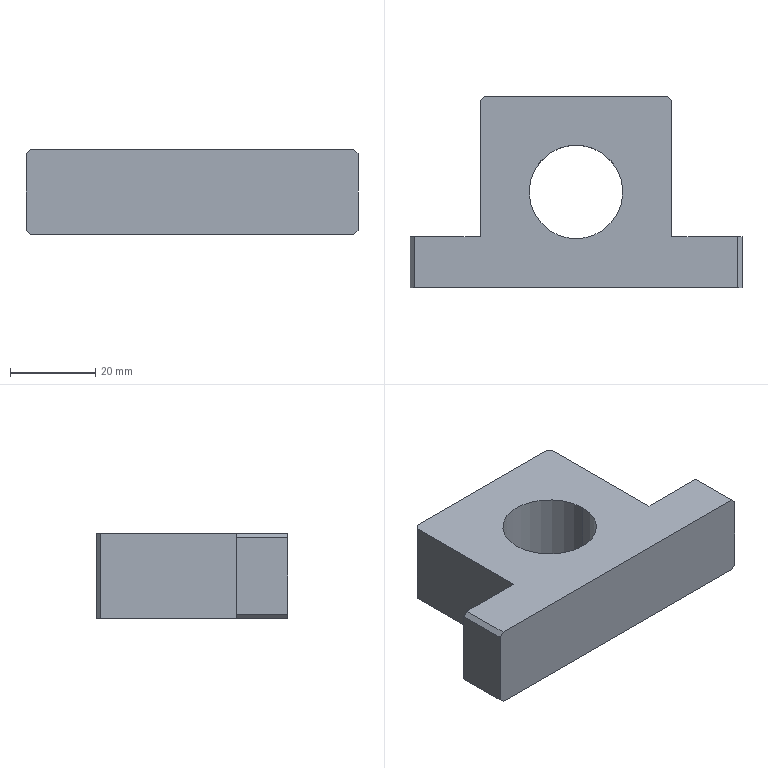Part | STEP file | 001-003-Shaft storage cylinder mounting seat | 1 solid | 18 faces | box 78 x 45 x 20 mm | volume 40773 mm3 | plane 16 | cylinder 2 | commonest cylinder face diameters 22 x2
STEP:
#1=CARTESIAN_POINT('',(0.,0.,0.));
#2=DIRECTION('',(0.,0.,1.));
#3=DIRECTION('',(1.,0.,0.));
#4=AXIS2_PLACEMENT_3D('',#1,#2,#3);
#5=CARTESIAN_POINT('',(11.,16.5,0.));
#6=VERTEX_POINT('',#5);
#7=CARTESIAN_POINT('',(11.,16.5,20.));
#8=VERTEX_POINT('',#7);
#9=CARTESIAN_POINT('',(11.,16.5,0.));
#10=DIRECTION('',(0.,0.,1.));
#11=VECTOR('',#10,1.);
#12=LINE('',#9,#11);
#13=CARTESIAN_POINT('',(0.,16.5,0.));
#14=DIRECTION('',(0.,0.,1.));
#15=DIRECTION('',(1.,0.,0.));
#16=AXIS2_PLACEMENT_3D('',#13,#14,#15);
#17=CYLINDRICAL_SURFACE('',#16,11.);
#18=CARTESIAN_POINT('',(6.283,0.));
#19=DIRECTION('',(0.,1.));
#20=VECTOR('',#19,1.);
#21=LINE('',#18,#20);
#22=(GEOMETRIC_REPRESENTATION_CONTEXT(2)PARAMETRIC_REPRESENTATION_CONTEXT()REPRESENTATION_CONTEXT('',''));
#23=DEFINITIONAL_REPRESENTATION('',(#21),#22);
#24=PCURVE('',#17,#23);
#25=CARTESIAN_POINT('',(0.,16.5,0.));
#26=DIRECTION('',(0.,0.,1.));
#27=DIRECTION('',(1.,0.,0.));
#28=AXIS2_PLACEMENT_3D('',#25,#26,#27);
#29=CYLINDRICAL_SURFACE('',#28,11.);
#30=CARTESIAN_POINT('',(0.,0.));
#31=DIRECTION('',(0.,1.));
#32=VECTOR('',#31,1.);
#33=LINE('',#30,#32);
#34=(GEOMETRIC_REPRESENTATION_CONTEXT(2)PARAMETRIC_REPRESENTATION_CONTEXT()REPRESENTATION_CONTEXT('',''));
#35=DEFINITIONAL_REPRESENTATION('',(#33),#34);
#36=PCURVE('',#29,#35);
#37=SURFACE_CURVE('',#12,(#24,#36),.PCURVE_S1.);
#38=EDGE_CURVE('',#6,#8,#37,.T.);
#39=ORIENTED_EDGE('',*,*,#38,.T.);
#40=CARTESIAN_POINT('',(-11.,16.5,20.));
#41=VERTEX_POINT('',#40);
#42=CARTESIAN_POINT('',(0.,16.5,20.));
#43=DIRECTION('',(0.,0.,1.));
#44=DIRECTION('',(1.,0.,0.));
#45=AXIS2_PLACEMENT_3D('',#42,#43,#44);
#46=CIRCLE('',#45,11.);
#47=CARTESIAN_POINT('',(0.,20.));
#48=DIRECTION('',(1.,0.));
#49=VECTOR('',#48,1.);
#50=LINE('',#47,#49);
#51=(GEOMETRIC_REPRESENTATION_CONTEXT(2)PARAMETRIC_REPRESENTATION_CONTEXT()REPRESENTATION_CONTEXT('',''));
#52=DEFINITIONAL_REPRESENTATION('',(#50),#51);
#53=PCURVE('',#17,#52);
#54=CARTESIAN_POINT('',(0.,0.,20.));
#55=DIRECTION('',(0.,0.,1.));
#56=DIRECTION('',(1.,0.,0.));
#57=AXIS2_PLACEMENT_3D('',#54,#55,#56);
#58=PLANE('',#57);
#59=CARTESIAN_POINT('',(0.,16.5));
#60=DIRECTION('',(1.,0.));
#61=AXIS2_PLACEMENT_2D('',#59,#60);
#62=CIRCLE('',#61,11.);
#63=(GEOMETRIC_REPRESENTATION_CONTEXT(2)PARAMETRIC_REPRESENTATION_CONTEXT()REPRESENTATION_CONTEXT('',''));
#64=DEFINITIONAL_REPRESENTATION('',(#62),#63);
#65=PCURVE('',#58,#64);
#66=SURFACE_CURVE('',#46,(#53,#65),.PCURVE_S1.);
#67=EDGE_CURVE('',#41,#8,#66,.T.);
#68=ORIENTED_EDGE('',*,*,#67,.F.);
#69=CARTESIAN_POINT('',(-11.,16.5,0.));
#70=VERTEX_POINT('',#69);
#71=CARTESIAN_POINT('',(-11.,16.5,0.));
#72=DIRECTION('',(0.,0.,1.));
#73=VECTOR('',#72,1.);
#74=LINE('',#71,#73);
#75=CARTESIAN_POINT('',(3.142,0.));
#76=DIRECTION('',(0.,1.));
#77=VECTOR('',#76,1.);
#78=LINE('',#75,#77);
#79=(GEOMETRIC_REPRESENTATION_CONTEXT(2)PARAMETRIC_REPRESENTATION_CONTEXT()REPRESENTATION_CONTEXT('',''));
#80=DEFINITIONAL_REPRESENTATION('',(#78),#79);
#81=PCURVE('',#17,#80);
#82=CARTESIAN_POINT('',(3.142,0.));
#83=DIRECTION('',(0.,1.));
#84=VECTOR('',#83,1.);
#85=LINE('',#82,#84);
#86=(GEOMETRIC_REPRESENTATION_CONTEXT(2)PARAMETRIC_REPRESENTATION_CONTEXT()REPRESENTATION_CONTEXT('',''));
#87=DEFINITIONAL_REPRESENTATION('',(#85),#86);
#88=PCURVE('',#29,#87);
#89=SURFACE_CURVE('',#74,(#81,#88),.PCURVE_S1.);
#90=EDGE_CURVE('',#70,#41,#89,.T.);
#91=ORIENTED_EDGE('',*,*,#90,.F.);
#92=CARTESIAN_POINT('',(0.,16.5,0.));
#93=DIRECTION('',(0.,0.,1.));
#94=DIRECTION('',(1.,0.,0.));
#95=AXIS2_PLACEMENT_3D('',#92,#93,#94);
#96=CIRCLE('',#95,11.);
#97=CARTESIAN_POINT('',(0.,0.));
#98=DIRECTION('',(1.,0.));
#99=VECTOR('',#98,1.);
#100=LINE('',#97,#99);
#101=(GEOMETRIC_REPRESENTATION_CONTEXT(2)PARAMETRIC_REPRESENTATION_CONTEXT()REPRESENTATION_CONTEXT('',''));
#102=DEFINITIONAL_REPRESENTATION('',(#100),#101);
#103=PCURVE('',#17,#102);
#104=CARTESIAN_POINT('',(0.,0.,0.));
#105=DIRECTION('',(0.,0.,1.));
#106=DIRECTION('',(1.,0.,0.));
#107=AXIS2_PLACEMENT_3D('',#104,#105,#106);
#108=PLANE('',#107);
#109=CARTESIAN_POINT('',(0.,16.5));
#110=DIRECTION('',(1.,0.));
#111=AXIS2_PLACEMENT_2D('',#109,#110);
#112=CIRCLE('',#111,11.);
#113=(GEOMETRIC_REPRESENTATION_CONTEXT(2)PARAMETRIC_REPRESENTATION_CONTEXT()REPRESENTATION_CONTEXT('',''));
#114=DEFINITIONAL_REPRESENTATION('',(#112),#113);
#115=PCURVE('',#108,#114);
#116=SURFACE_CURVE('',#96,(#103,#115),.PCURVE_S1.);
#117=EDGE_CURVE('',#70,#6,#116,.T.);
#118=ORIENTED_EDGE('',*,*,#117,.T.);
#119=EDGE_LOOP('',(#39,#68,#91,#118));
#120=FACE_BOUND('',#119,.F.);
#121=ADVANCED_FACE('',(#120),#17,.F.);
#122=CARTESIAN_POINT('',(39.,6.,19.));
#123=VERTEX_POINT('',#122);
#124=CARTESIAN_POINT('',(39.,6.,1.));
#125=VERTEX_POINT('',#124);
#126=CARTESIAN_POINT('',(39.,6.,20.));
#127=DIRECTION('',(0.,0.,-1.));
#128=VECTOR('',#127,1.);
#129=LINE('',#126,#128);
#130=CARTESIAN_POINT('',(22.5,6.,20.));
#131=DIRECTION('',(0.,-1.,0.));
#132=DIRECTION('',(1.,0.,0.));
#133=AXIS2_PLACEMENT_3D('',#130,#131,#132);
#134=PLANE('',#133);
#135=CARTESIAN_POINT('',(16.5,0.));
#136=DIRECTION('',(0.,-1.));
#137=VECTOR('',#136,1.);
#138=LINE('',#135,#137);
#139=(GEOMETRIC_REPRESENTATION_CONTEXT(2)PARAMETRIC_REPRESENTATION_CONTEXT()REPRESENTATION_CONTEXT('',''));
#140=DEFINITIONAL_REPRESENTATION('',(#138),#139);
#141=PCURVE('',#134,#140);
#142=CARTESIAN_POINT('',(39.,-6.,20.));
#143=DIRECTION('',(-1.,0.,0.));
#144=DIRECTION('',(0.,0.,1.));
#145=AXIS2_PLACEMENT_3D('',#142,#143,#144);
#146=PLANE('',#145);
#147=CARTESIAN_POINT('',(0.,12.));
#148=DIRECTION('',(-1.,0.));
#149=VECTOR('',#148,1.);
#150=LINE('',#147,#149);
#151=(GEOMETRIC_REPRESENTATION_CONTEXT(2)PARAMETRIC_REPRESENTATION_CONTEXT()REPRESENTATION_CONTEXT('',''));
#152=DEFINITIONAL_REPRESENTATION('',(#150),#151);
#153=PCURVE('',#146,#152);
#154=SURFACE_CURVE('',#129,(#141,#153),.PCURVE_S1.);
#155=EDGE_CURVE('',#123,#125,#154,.T.);
#156=ORIENTED_EDGE('',*,*,#155,.T.);
#157=CARTESIAN_POINT('',(38.,6.,0.));
#158=VERTEX_POINT('',#157);
#159=CARTESIAN_POINT('',(39.,6.,1.));
#160=DIRECTION('',(-0.7071,0.,-0.7071));
#161=VECTOR('',#160,1.);
#162=LINE('',#159,#161);
#163=CARTESIAN_POINT('',(16.5,-19.));
#164=DIRECTION('',(-0.7071,-0.7071));
#165=VECTOR('',#164,1.);
#166=LINE('',#163,#165);
#167=(GEOMETRIC_REPRESENTATION_CONTEXT(2)PARAMETRIC_REPRESENTATION_CONTEXT()REPRESENTATION_CONTEXT('',''));
#168=DEFINITIONAL_REPRESENTATION('',(#166),#167);
#169=PCURVE('',#134,#168);
#170=CARTESIAN_POINT('',(39.,-6.,1.));
#171=DIRECTION('',(-0.7071,0.,0.7071));
#172=DIRECTION('',(0.,1.,0.));
#173=AXIS2_PLACEMENT_3D('',#170,#171,#172);
#174=PLANE('',#173);
#175=CARTESIAN_POINT('',(12.,0.));
#176=DIRECTION('',(0.,1.));
#177=VECTOR('',#176,1.);
#178=LINE('',#175,#177);
#179=(GEOMETRIC_REPRESENTATION_CONTEXT(2)PARAMETRIC_REPRESENTATION_CONTEXT()REPRESENTATION_CONTEXT('',''));
#180=DEFINITIONAL_REPRESENTATION('',(#178),#179);
#181=PCURVE('',#174,#180);
#182=SURFACE_CURVE('',#162,(#169,#181),.PCURVE_S1.);
#183=EDGE_CURVE('',#125,#158,#182,.T.);
#184=ORIENTED_EDGE('',*,*,#183,.T.);
#185=CARTESIAN_POINT('',(22.5,6.,0.));
#186=VERTEX_POINT('',#185);
#187=CARTESIAN_POINT('',(22.5,6.,0.));
#188=DIRECTION('',(-1.,0.,0.));
#189=VECTOR('',#188,1.);
#190=LINE('',#187,#189);
#191=CARTESIAN_POINT('',(0.,-20.));
#192=DIRECTION('',(-1.,0.));
#193=VECTOR('',#192,1.);
#194=LINE('',#191,#193);
#195=(GEOMETRIC_REPRESENTATION_CONTEXT(2)PARAMETRIC_REPRESENTATION_CONTEXT()REPRESENTATION_CONTEXT('',''));
#196=DEFINITIONAL_REPRESENTATION('',(#194),#195);
#197=PCURVE('',#134,#196);
#198=CARTESIAN_POINT('',(22.5,6.));
#199=DIRECTION('',(-1.,0.));
#200=VECTOR('',#199,1.);
#201=LINE('',#198,#200);
#202=(GEOMETRIC_REPRESENTATION_CONTEXT(2)PARAMETRIC_REPRESENTATION_CONTEXT()REPRESENTATION_CONTEXT('',''));
#203=DEFINITIONAL_REPRESENTATION('',(#201),#202);
#204=PCURVE('',#108,#203);
#205=SURFACE_CURVE('',#190,(#197,#204),.PCURVE_S1.);
#206=EDGE_CURVE('',#158,#186,#205,.T.);
#207=ORIENTED_EDGE('',*,*,#206,.T.);
#208=CARTESIAN_POINT('',(22.5,6.,20.));
#209=VERTEX_POINT('',#208);
#210=CARTESIAN_POINT('',(22.5,6.,20.));
#211=DIRECTION('',(0.,0.,-1.));
#212=VECTOR('',#211,1.);
#213=LINE('',#210,#212);
#214=CARTESIAN_POINT('',(0.,0.));
#215=DIRECTION('',(0.,-1.));
#216=VECTOR('',#215,1.);
#217=LINE('',#214,#216);
#218=(GEOMETRIC_REPRESENTATION_CONTEXT(2)PARAMETRIC_REPRESENTATION_CONTEXT()REPRESENTATION_CONTEXT('',''));
#219=DEFINITIONAL_REPRESENTATION('',(#217),#218);
#220=PCURVE('',#134,#219);
#221=CARTESIAN_POINT('',(22.5,6.,20.));
#222=DIRECTION('',(-1.,0.,0.));
#223=DIRECTION('',(0.,-1.,0.));
#224=AXIS2_PLACEMENT_3D('',#221,#222,#223);
#225=PLANE('',#224);
#226=CARTESIAN_POINT('',(0.,0.));
#227=DIRECTION('',(0.,-1.));
#228=VECTOR('',#227,1.);
#229=LINE('',#226,#228);
#230=(GEOMETRIC_REPRESENTATION_CONTEXT(2)PARAMETRIC_REPRESENTATION_CONTEXT()REPRESENTATION_CONTEXT('',''));
#231=DEFINITIONAL_REPRESENTATION('',(#229),#230);
#232=PCURVE('',#225,#231);
#233=SURFACE_CURVE('',#213,(#220,#232),.PCURVE_S1.);
#234=EDGE_CURVE('',#209,#186,#233,.T.);
#235=ORIENTED_EDGE('',*,*,#234,.F.);
#236=CARTESIAN_POINT('',(38.,6.,20.));
#237=VERTEX_POINT('',#236);
#238=CARTESIAN_POINT('',(22.5,6.,20.));
#239=DIRECTION('',(-1.,0.,0.));
#240=VECTOR('',#239,1.);
#241=LINE('',#238,#240);
#242=CARTESIAN_POINT('',(0.,0.));
#243=DIRECTION('',(-1.,0.));
#244=VECTOR('',#243,1.);
#245=LINE('',#242,#244);
#246=(GEOMETRIC_REPRESENTATION_CONTEXT(2)PARAMETRIC_REPRESENTATION_CONTEXT()REPRESENTATION_CONTEXT('',''));
#247=DEFINITIONAL_REPRESENTATION('',(#245),#246);
#248=PCURVE('',#134,#247);
#249=CARTESIAN_POINT('',(22.5,6.));
#250=DIRECTION('',(-1.,0.));
#251=VECTOR('',#250,1.);
#252=LINE('',#249,#251);
#253=(GEOMETRIC_REPRESENTATION_CONTEXT(2)PARAMETRIC_REPRESENTATION_CONTEXT()REPRESENTATION_CONTEXT('',''));
#254=DEFINITIONAL_REPRESENTATION('',(#252),#253);
#255=PCURVE('',#58,#254);
#256=SURFACE_CURVE('',#241,(#248,#255),.PCURVE_S1.);
#257=EDGE_CURVE('',#237,#209,#256,.T.);
#258=ORIENTED_EDGE('',*,*,#257,.F.);
#259=CARTESIAN_POINT('',(38.,6.,20.));
#260=DIRECTION('',(0.7071,0.,-0.7071));
#261=VECTOR('',#260,1.);
#262=LINE('',#259,#261);
#263=CARTESIAN_POINT('',(15.5,0.));
#264=DIRECTION('',(0.7071,-0.7071));
#265=VECTOR('',#264,1.);
#266=LINE('',#263,#265);
#267=(GEOMETRIC_REPRESENTATION_CONTEXT(2)PARAMETRIC_REPRESENTATION_CONTEXT()REPRESENTATION_CONTEXT('',''));
#268=DEFINITIONAL_REPRESENTATION('',(#266),#267);
#269=PCURVE('',#134,#268);
#270=CARTESIAN_POINT('',(38.,0.,20.));
#271=DIRECTION('',(0.7071,0.,0.7071));
#272=DIRECTION('',(0.,-1.,0.));
#273=AXIS2_PLACEMENT_3D('',#270,#271,#272);
#274=PLANE('',#273);
#275=CARTESIAN_POINT('',(-6.,0.));
#276=DIRECTION('',(0.,1.));
#277=VECTOR('',#276,1.);
#278=LINE('',#275,#277);
#279=(GEOMETRIC_REPRESENTATION_CONTEXT(2)PARAMETRIC_REPRESENTATION_CONTEXT()REPRESENTATION_CONTEXT('',''));
#280=DEFINITIONAL_REPRESENTATION('',(#278),#279);
#281=PCURVE('',#274,#280);
#282=SURFACE_CURVE('',#262,(#269,#281),.PCURVE_S1.);
#283=EDGE_CURVE('',#237,#123,#282,.T.);
#284=ORIENTED_EDGE('',*,*,#283,.T.);
#285=EDGE_LOOP('',(#156,#184,#207,#235,#258,#284));
#286=FACE_BOUND('',#285,.T.);
#287=ADVANCED_FACE('',(#286),#134,.F.);
#288=CARTESIAN_POINT('',(22.5,38.,0.));
#289=VERTEX_POINT('',#288);
#290=CARTESIAN_POINT('',(22.5,6.,0.));
#291=DIRECTION('',(0.,1.,0.));
#292=VECTOR('',#291,1.);
#293=LINE('',#290,#292);
#294=CARTESIAN_POINT('',(0.,-20.));
#295=DIRECTION('',(-1.,0.));
#296=VECTOR('',#295,1.);
#297=LINE('',#294,#296);
#298=(GEOMETRIC_REPRESENTATION_CONTEXT(2)PARAMETRIC_REPRESENTATION_CONTEXT()REPRESENTATION_CONTEXT('',''));
#299=DEFINITIONAL_REPRESENTATION('',(#297),#298);
#300=PCURVE('',#225,#299);
#301=CARTESIAN_POINT('',(22.5,6.));
#302=DIRECTION('',(0.,1.));
#303=VECTOR('',#302,1.);
#304=LINE('',#301,#303);
#305=(GEOMETRIC_REPRESENTATION_CONTEXT(2)PARAMETRIC_REPRESENTATION_CONTEXT()REPRESENTATION_CONTEXT('',''));
#306=DEFINITIONAL_REPRESENTATION('',(#304),#305);
#307=PCURVE('',#108,#306);
#308=SURFACE_CURVE('',#293,(#300,#307),.PCURVE_S1.);
#309=EDGE_CURVE('',#186,#289,#308,.T.);
#310=ORIENTED_EDGE('',*,*,#309,.T.);
#311=CARTESIAN_POINT('',(22.5,38.,20.));
#312=VERTEX_POINT('',#311);
#313=CARTESIAN_POINT('',(22.5,38.,20.));
#314=DIRECTION('',(0.,0.,1.));
#315=VECTOR('',#314,1.);
#316=LINE('',#313,#315);
#317=CARTESIAN_POINT('',(-32.,0.));
#318=DIRECTION('',(0.,1.));
#319=VECTOR('',#318,1.);
#320=LINE('',#317,#319);
#321=(GEOMETRIC_REPRESENTATION_CONTEXT(2)PARAMETRIC_REPRESENTATION_CONTEXT()REPRESENTATION_CONTEXT('',''));
#322=DEFINITIONAL_REPRESENTATION('',(#320),#321);
#323=PCURVE('',#225,#322);
#324=CARTESIAN_POINT('',(21.5,39.,20.));
#325=DIRECTION('',(-0.7071,-0.7071,0.));
#326=DIRECTION('',(0.,0.,-1.));
#327=AXIS2_PLACEMENT_3D('',#324,#325,#326);
#328=PLANE('',#327);
#329=CARTESIAN_POINT('',(0.,1.414));
#330=DIRECTION('',(-1.,0.));
#331=VECTOR('',#330,1.);
#332=LINE('',#329,#331);
#333=(GEOMETRIC_REPRESENTATION_CONTEXT(2)PARAMETRIC_REPRESENTATION_CONTEXT()REPRESENTATION_CONTEXT('',''));
#334=DEFINITIONAL_REPRESENTATION('',(#332),#333);
#335=PCURVE('',#328,#334);
#336=SURFACE_CURVE('',#316,(#323,#335),.PCURVE_S1.);
#337=EDGE_CURVE('',#289,#312,#336,.T.);
#338=ORIENTED_EDGE('',*,*,#337,.T.);
#339=CARTESIAN_POINT('',(22.5,6.,20.));
#340=DIRECTION('',(0.,1.,0.));
#341=VECTOR('',#340,1.);
#342=LINE('',#339,#341);
#343=CARTESIAN_POINT('',(0.,0.));
#344=DIRECTION('',(-1.,0.));
#345=VECTOR('',#344,1.);
#346=LINE('',#343,#345);
#347=(GEOMETRIC_REPRESENTATION_CONTEXT(2)PARAMETRIC_REPRESENTATION_CONTEXT()REPRESENTATION_CONTEXT('',''));
#348=DEFINITIONAL_REPRESENTATION('',(#346),#347);
#349=PCURVE('',#225,#348);
#350=CARTESIAN_POINT('',(22.5,6.));
#351=DIRECTION('',(0.,1.));
#352=VECTOR('',#351,1.);
#353=LINE('',#350,#352);
#354=(GEOMETRIC_REPRESENTATION_CONTEXT(2)PARAMETRIC_REPRESENTATION_CONTEXT()REPRESENTATION_CONTEXT('',''));
#355=DEFINITIONAL_REPRESENTATION('',(#353),#354);
#356=PCURVE('',#58,#355);
#357=SURFACE_CURVE('',#342,(#349,#356),.PCURVE_S1.);
#358=EDGE_CURVE('',#209,#312,#357,.T.);
#359=ORIENTED_EDGE('',*,*,#358,.F.);
#360=ORIENTED_EDGE('',*,*,#234,.T.);
#361=EDGE_LOOP('',(#310,#338,#359,#360));
#362=FACE_BOUND('',#361,.T.);
#363=ADVANCED_FACE('',(#362),#225,.F.);
#364=CARTESIAN_POINT('',(21.5,39.,20.));
#365=VERTEX_POINT('',#364);
#366=CARTESIAN_POINT('',(-21.5,39.,20.));
#367=VERTEX_POINT('',#366);
#368=CARTESIAN_POINT('',(-22.5,39.,20.));
#369=DIRECTION('',(-1.,0.,0.));
#370=VECTOR('',#369,1.);
#371=LINE('',#368,#370);
#372=CARTESIAN_POINT('',(-22.5,39.,20.));
#373=DIRECTION('',(0.,-1.,0.));
#374=DIRECTION('',(1.,0.,0.));
#375=AXIS2_PLACEMENT_3D('',#372,#373,#374);
#376=PLANE('',#375);
#377=CARTESIAN_POINT('',(0.,0.));
#378=DIRECTION('',(-1.,0.));
#379=VECTOR('',#378,1.);
#380=LINE('',#377,#379);
#381=(GEOMETRIC_REPRESENTATION_CONTEXT(2)PARAMETRIC_REPRESENTATION_CONTEXT()REPRESENTATION_CONTEXT('',''));
#382=DEFINITIONAL_REPRESENTATION('',(#380),#381);
#383=PCURVE('',#376,#382);
#384=CARTESIAN_POINT('',(-22.5,39.));
#385=DIRECTION('',(-1.,0.));
#386=VECTOR('',#385,1.);
#387=LINE('',#384,#386);
#388=(GEOMETRIC_REPRESENTATION_CONTEXT(2)PARAMETRIC_REPRESENTATION_CONTEXT()REPRESENTATION_CONTEXT('',''));
#389=DEFINITIONAL_REPRESENTATION('',(#387),#388);
#390=PCURVE('',#58,#389);
#391=SURFACE_CURVE('',#371,(#383,#390),.PCURVE_S1.);
#392=EDGE_CURVE('',#365,#367,#391,.T.);
#393=ORIENTED_EDGE('',*,*,#392,.F.);
#394=CARTESIAN_POINT('',(21.5,39.,0.));
#395=VERTEX_POINT('',#394);
#396=CARTESIAN_POINT('',(21.5,39.,20.));
#397=DIRECTION('',(0.,0.,-1.));
#398=VECTOR('',#397,1.);
#399=LINE('',#396,#398);
#400=CARTESIAN_POINT('',(44.,0.));
#401=DIRECTION('',(0.,-1.));
#402=VECTOR('',#401,1.);
#403=LINE('',#400,#402);
#404=(GEOMETRIC_REPRESENTATION_CONTEXT(2)PARAMETRIC_REPRESENTATION_CONTEXT()REPRESENTATION_CONTEXT('',''));
#405=DEFINITIONAL_REPRESENTATION('',(#403),#404);
#406=PCURVE('',#376,#405);
#407=CARTESIAN_POINT('',(0.,0.));
#408=DIRECTION('',(1.,0.));
#409=VECTOR('',#408,1.);
#410=LINE('',#407,#409);
#411=(GEOMETRIC_REPRESENTATION_CONTEXT(2)PARAMETRIC_REPRESENTATION_CONTEXT()REPRESENTATION_CONTEXT('',''));
#412=DEFINITIONAL_REPRESENTATION('',(#410),#411);
#413=PCURVE('',#328,#412);
#414=SURFACE_CURVE('',#399,(#406,#413),.PCURVE_S1.);
#415=EDGE_CURVE('',#365,#395,#414,.T.);
#416=ORIENTED_EDGE('',*,*,#415,.T.);
#417=CARTESIAN_POINT('',(-21.5,39.,0.));
#418=VERTEX_POINT('',#417);
#419=CARTESIAN_POINT('',(-22.5,39.,0.));
#420=DIRECTION('',(-1.,0.,0.));
#421=VECTOR('',#420,1.);
#422=LINE('',#419,#421);
#423=CARTESIAN_POINT('',(0.,-20.));
#424=DIRECTION('',(-1.,0.));
#425=VECTOR('',#424,1.);
#426=LINE('',#423,#425);
#427=(GEOMETRIC_REPRESENTATION_CONTEXT(2)PARAMETRIC_REPRESENTATION_CONTEXT()REPRESENTATION_CONTEXT('',''));
#428=DEFINITIONAL_REPRESENTATION('',(#426),#427);
#429=PCURVE('',#376,#428);
#430=CARTESIAN_POINT('',(-22.5,39.));
#431=DIRECTION('',(-1.,0.));
#432=VECTOR('',#431,1.);
#433=LINE('',#430,#432);
#434=(GEOMETRIC_REPRESENTATION_CONTEXT(2)PARAMETRIC_REPRESENTATION_CONTEXT()REPRESENTATION_CONTEXT('',''));
#435=DEFINITIONAL_REPRESENTATION('',(#433),#434);
#436=PCURVE('',#108,#435);
#437=SURFACE_CURVE('',#422,(#429,#436),.PCURVE_S1.);
#438=EDGE_CURVE('',#395,#418,#437,.T.);
#439=ORIENTED_EDGE('',*,*,#438,.T.);
#440=CARTESIAN_POINT('',(-21.5,39.,20.));
#441=DIRECTION('',(0.,0.,1.));
#442=VECTOR('',#441,1.);
#443=LINE('',#440,#442);
#444=CARTESIAN_POINT('',(1.,0.));
#445=DIRECTION('',(0.,1.));
#446=VECTOR('',#445,1.);
#447=LINE('',#444,#446);
#448=(GEOMETRIC_REPRESENTATION_CONTEXT(2)PARAMETRIC_REPRESENTATION_CONTEXT()REPRESENTATION_CONTEXT('',''));
#449=DEFINITIONAL_REPRESENTATION('',(#447),#448);
#450=PCURVE('',#376,#449);
#451=CARTESIAN_POINT('',(-22.5,38.,20.));
#452=DIRECTION('',(0.7071,-0.7071,0.));
#453=DIRECTION('',(0.,0.,-1.));
#454=AXIS2_PLACEMENT_3D('',#451,#452,#453);
#455=PLANE('',#454);
#456=CARTESIAN_POINT('',(0.,1.414));
#457=DIRECTION('',(-1.,0.));
#458=VECTOR('',#457,1.);
#459=LINE('',#456,#458);
#460=(GEOMETRIC_REPRESENTATION_CONTEXT(2)PARAMETRIC_REPRESENTATION_CONTEXT()REPRESENTATION_CONTEXT('',''));
#461=DEFINITIONAL_REPRESENTATION('',(#459),#460);
#462=PCURVE('',#455,#461);
#463=SURFACE_CURVE('',#443,(#450,#462),.PCURVE_S1.);
#464=EDGE_CURVE('',#418,#367,#463,.T.);
#465=ORIENTED_EDGE('',*,*,#464,.T.);
#466=EDGE_LOOP('',(#393,#416,#439,#465));
#467=FACE_BOUND('',#466,.T.);
#468=ADVANCED_FACE('',(#467),#376,.F.);
#469=CARTESIAN_POINT('',(-22.5,38.,20.));
#470=VERTEX_POINT('',#469);
#471=CARTESIAN_POINT('',(-22.5,6.,20.));
#472=VERTEX_POINT('',#471);
#473=CARTESIAN_POINT('',(-22.5,6.,20.));
#474=DIRECTION('',(0.,-1.,0.));
#475=VECTOR('',#474,1.);
#476=LINE('',#473,#475);
#477=CARTESIAN_POINT('',(-22.5,6.,20.));
#478=DIRECTION('',(1.,0.,0.));
#479=DIRECTION('',(0.,0.,-1.));
#480=AXIS2_PLACEMENT_3D('',#477,#478,#479);
#481=PLANE('',#480);
#482=CARTESIAN_POINT('',(0.,0.));
#483=DIRECTION('',(0.,-1.));
#484=VECTOR('',#483,1.);
#485=LINE('',#482,#484);
#486=(GEOMETRIC_REPRESENTATION_CONTEXT(2)PARAMETRIC_REPRESENTATION_CONTEXT()REPRESENTATION_CONTEXT('',''));
#487=DEFINITIONAL_REPRESENTATION('',(#485),#486);
#488=PCURVE('',#481,#487);
#489=CARTESIAN_POINT('',(-22.5,6.));
#490=DIRECTION('',(0.,-1.));
#491=VECTOR('',#490,1.);
#492=LINE('',#489,#491);
#493=(GEOMETRIC_REPRESENTATION_CONTEXT(2)PARAMETRIC_REPRESENTATION_CONTEXT()REPRESENTATION_CONTEXT('',''));
#494=DEFINITIONAL_REPRESENTATION('',(#492),#493);
#495=PCURVE('',#58,#494);
#496=SURFACE_CURVE('',#476,(#488,#495),.PCURVE_S1.);
#497=EDGE_CURVE('',#470,#472,#496,.T.);
#498=ORIENTED_EDGE('',*,*,#497,.F.);
#499=CARTESIAN_POINT('',(-22.5,38.,0.));
#500=VERTEX_POINT('',#499);
#501=CARTESIAN_POINT('',(-22.5,38.,20.));
#502=DIRECTION('',(0.,0.,-1.));
#503=VECTOR('',#502,1.);
#504=LINE('',#501,#503);
#505=CARTESIAN_POINT('',(0.,32.));
#506=DIRECTION('',(1.,0.));
#507=VECTOR('',#506,1.);
#508=LINE('',#505,#507);
#509=(GEOMETRIC_REPRESENTATION_CONTEXT(2)PARAMETRIC_REPRESENTATION_CONTEXT()REPRESENTATION_CONTEXT('',''));
#510=DEFINITIONAL_REPRESENTATION('',(#508),#509);
#511=PCURVE('',#481,#510);
#512=CARTESIAN_POINT('',(0.,0.));
#513=DIRECTION('',(1.,0.));
#514=VECTOR('',#513,1.);
#515=LINE('',#512,#514);
#516=(GEOMETRIC_REPRESENTATION_CONTEXT(2)PARAMETRIC_REPRESENTATION_CONTEXT()REPRESENTATION_CONTEXT('',''));
#517=DEFINITIONAL_REPRESENTATION('',(#515),#516);
#518=PCURVE('',#455,#517);
#519=SURFACE_CURVE('',#504,(#511,#518),.PCURVE_S1.);
#520=EDGE_CURVE('',#470,#500,#519,.T.);
#521=ORIENTED_EDGE('',*,*,#520,.T.);
#522=CARTESIAN_POINT('',(-22.5,6.,0.));
#523=VERTEX_POINT('',#522);
#524=CARTESIAN_POINT('',(-22.5,6.,0.));
#525=DIRECTION('',(0.,-1.,0.));
#526=VECTOR('',#525,1.);
#527=LINE('',#524,#526);
#528=CARTESIAN_POINT('',(20.,0.));
#529=DIRECTION('',(0.,-1.));
#530=VECTOR('',#529,1.);
#531=LINE('',#528,#530);
#532=(GEOMETRIC_REPRESENTATION_CONTEXT(2)PARAMETRIC_REPRESENTATION_CONTEXT()REPRESENTATION_CONTEXT('',''));
#533=DEFINITIONAL_REPRESENTATION('',(#531),#532);
#534=PCURVE('',#481,#533);
#535=CARTESIAN_POINT('',(-22.5,6.));
#536=DIRECTION('',(0.,-1.));
#537=VECTOR('',#536,1.);
#538=LINE('',#535,#537);
#539=(GEOMETRIC_REPRESENTATION_CONTEXT(2)PARAMETRIC_REPRESENTATION_CONTEXT()REPRESENTATION_CONTEXT('',''));
#540=DEFINITIONAL_REPRESENTATION('',(#538),#539);
#541=PCURVE('',#108,#540);
#542=SURFACE_CURVE('',#527,(#534,#541),.PCURVE_S1.);
#543=EDGE_CURVE('',#500,#523,#542,.T.);
#544=ORIENTED_EDGE('',*,*,#543,.T.);
#545=CARTESIAN_POINT('',(-22.5,6.,20.));
#546=DIRECTION('',(0.,0.,-1.));
#547=VECTOR('',#546,1.);
#548=LINE('',#545,#547);
#549=CARTESIAN_POINT('',(0.,0.));
#550=DIRECTION('',(1.,0.));
#551=VECTOR('',#550,1.);
#552=LINE('',#549,#551);
#553=(GEOMETRIC_REPRESENTATION_CONTEXT(2)PARAMETRIC_REPRESENTATION_CONTEXT()REPRESENTATION_CONTEXT('',''));
#554=DEFINITIONAL_REPRESENTATION('',(#552),#553);
#555=PCURVE('',#481,#554);
#556=CARTESIAN_POINT('',(-39.,6.,20.));
#557=DIRECTION('',(0.,-1.,0.));
#558=DIRECTION('',(1.,0.,0.));
#559=AXIS2_PLACEMENT_3D('',#556,#557,#558);
#560=PLANE('',#559);
#561=CARTESIAN_POINT('',(16.5,0.));
#562=DIRECTION('',(0.,-1.));
#563=VECTOR('',#562,1.);
#564=LINE('',#561,#563);
#565=(GEOMETRIC_REPRESENTATION_CONTEXT(2)PARAMETRIC_REPRESENTATION_CONTEXT()REPRESENTATION_CONTEXT('',''));
#566=DEFINITIONAL_REPRESENTATION('',(#564),#565);
#567=PCURVE('',#560,#566);
#568=SURFACE_CURVE('',#548,(#555,#567),.PCURVE_S1.);
#569=EDGE_CURVE('',#472,#523,#568,.T.);
#570=ORIENTED_EDGE('',*,*,#569,.F.);
#571=EDGE_LOOP('',(#498,#521,#544,#570));
#572=FACE_BOUND('',#571,.T.);
#573=ADVANCED_FACE('',(#572),#481,.F.);
#574=CARTESIAN_POINT('',(-38.,6.,0.));
#575=VERTEX_POINT('',#574);
#576=CARTESIAN_POINT('',(-39.,6.,0.));
#577=DIRECTION('',(-1.,0.,0.));
#578=VECTOR('',#577,1.);
#579=LINE('',#576,#578);
#580=CARTESIAN_POINT('',(0.,-20.));
#581=DIRECTION('',(-1.,0.));
#582=VECTOR('',#581,1.);
#583=LINE('',#580,#582);
#584=(GEOMETRIC_REPRESENTATION_CONTEXT(2)PARAMETRIC_REPRESENTATION_CONTEXT()REPRESENTATION_CONTEXT('',''));
#585=DEFINITIONAL_REPRESENTATION('',(#583),#584);
#586=PCURVE('',#560,#585);
#587=CARTESIAN_POINT('',(-39.,6.));
#588=DIRECTION('',(-1.,0.));
#589=VECTOR('',#588,1.);
#590=LINE('',#587,#589);
#591=(GEOMETRIC_REPRESENTATION_CONTEXT(2)PARAMETRIC_REPRESENTATION_CONTEXT()REPRESENTATION_CONTEXT('',''));
#592=DEFINITIONAL_REPRESENTATION('',(#590),#591);
#593=PCURVE('',#108,#592);
#594=SURFACE_CURVE('',#579,(#586,#593),.PCURVE_S1.);
#595=EDGE_CURVE('',#523,#575,#594,.T.);
#596=ORIENTED_EDGE('',*,*,#595,.T.);
#597=CARTESIAN_POINT('',(-39.,6.,1.));
#598=VERTEX_POINT('',#597);
#599=CARTESIAN_POINT('',(-39.,6.,1.));
#600=DIRECTION('',(-0.7071,0.,0.7071));
#601=VECTOR('',#600,1.);
#602=LINE('',#599,#601);
#603=CARTESIAN_POINT('',(0.,-19.));
#604=DIRECTION('',(-0.7071,0.7071));
#605=VECTOR('',#604,1.);
#606=LINE('',#603,#605);
#607=(GEOMETRIC_REPRESENTATION_CONTEXT(2)PARAMETRIC_REPRESENTATION_CONTEXT()REPRESENTATION_CONTEXT('',''));
#608=DEFINITIONAL_REPRESENTATION('',(#606),#607);
#609=PCURVE('',#560,#608);
#610=CARTESIAN_POINT('',(-39.,-6.,1.));
#611=DIRECTION('',(0.7071,0.,0.7071));
#612=DIRECTION('',(0.,-1.,0.));
#613=AXIS2_PLACEMENT_3D('',#610,#611,#612);
#614=PLANE('',#613);
#615=CARTESIAN_POINT('',(-12.,0.));
#616=DIRECTION('',(0.,-1.));
#617=VECTOR('',#616,1.);
#618=LINE('',#615,#617);
#619=(GEOMETRIC_REPRESENTATION_CONTEXT(2)PARAMETRIC_REPRESENTATION_CONTEXT()REPRESENTATION_CONTEXT('',''));
#620=DEFINITIONAL_REPRESENTATION('',(#618),#619);
#621=PCURVE('',#614,#620);
#622=SURFACE_CURVE('',#602,(#609,#621),.PCURVE_S1.);
#623=EDGE_CURVE('',#575,#598,#622,.T.);
#624=ORIENTED_EDGE('',*,*,#623,.T.);
#625=CARTESIAN_POINT('',(-39.,6.,19.));
#626=VERTEX_POINT('',#625);
#627=CARTESIAN_POINT('',(-39.,6.,20.));
#628=DIRECTION('',(0.,0.,-1.));
#629=VECTOR('',#628,1.);
#630=LINE('',#627,#629);
#631=CARTESIAN_POINT('',(0.,0.));
#632=DIRECTION('',(0.,-1.));
#633=VECTOR('',#632,1.);
#634=LINE('',#631,#633);
#635=(GEOMETRIC_REPRESENTATION_CONTEXT(2)PARAMETRIC_REPRESENTATION_CONTEXT()REPRESENTATION_CONTEXT('',''));
#636=DEFINITIONAL_REPRESENTATION('',(#634),#635);
#637=PCURVE('',#560,#636);
#638=CARTESIAN_POINT('',(-39.,-6.,20.));
#639=DIRECTION('',(1.,0.,0.));
#640=DIRECTION('',(0.,0.,-1.));
#641=AXIS2_PLACEMENT_3D('',#638,#639,#640);
#642=PLANE('',#641);
#643=CARTESIAN_POINT('',(0.,12.));
#644=DIRECTION('',(1.,0.));
#645=VECTOR('',#644,1.);
#646=LINE('',#643,#645);
#647=(GEOMETRIC_REPRESENTATION_CONTEXT(2)PARAMETRIC_REPRESENTATION_CONTEXT()REPRESENTATION_CONTEXT('',''));
#648=DEFINITIONAL_REPRESENTATION('',(#646),#647);
#649=PCURVE('',#642,#648);
#650=SURFACE_CURVE('',#630,(#637,#649),.PCURVE_S1.);
#651=EDGE_CURVE('',#626,#598,#650,.T.);
#652=ORIENTED_EDGE('',*,*,#651,.F.);
#653=CARTESIAN_POINT('',(-38.,6.,20.));
#654=VERTEX_POINT('',#653);
#655=CARTESIAN_POINT('',(-38.,6.,20.));
#656=DIRECTION('',(0.7071,0.,0.7071));
#657=VECTOR('',#656,1.);
#658=LINE('',#655,#657);
#659=CARTESIAN_POINT('',(1.,0.));
#660=DIRECTION('',(0.7071,0.7071));
#661=VECTOR('',#660,1.);
#662=LINE('',#659,#661);
#663=(GEOMETRIC_REPRESENTATION_CONTEXT(2)PARAMETRIC_REPRESENTATION_CONTEXT()REPRESENTATION_CONTEXT('',''));
#664=DEFINITIONAL_REPRESENTATION('',(#662),#663);
#665=PCURVE('',#560,#664);
#666=CARTESIAN_POINT('',(-38.,0.,20.));
#667=DIRECTION('',(-0.7071,0.,0.7071));
#668=DIRECTION('',(0.,1.,0.));
#669=AXIS2_PLACEMENT_3D('',#666,#667,#668);
#670=PLANE('',#669);
#671=CARTESIAN_POINT('',(6.,0.));
#672=DIRECTION('',(0.,-1.));
#673=VECTOR('',#672,1.);
#674=LINE('',#671,#673);
#675=(GEOMETRIC_REPRESENTATION_CONTEXT(2)PARAMETRIC_REPRESENTATION_CONTEXT()REPRESENTATION_CONTEXT('',''));
#676=DEFINITIONAL_REPRESENTATION('',(#674),#675);
#677=PCURVE('',#670,#676);
#678=SURFACE_CURVE('',#658,(#665,#677),.PCURVE_S1.);
#679=EDGE_CURVE('',#626,#654,#678,.T.);
#680=ORIENTED_EDGE('',*,*,#679,.T.);
#681=CARTESIAN_POINT('',(-39.,6.,20.));
#682=DIRECTION('',(-1.,0.,0.));
#683=VECTOR('',#682,1.);
#684=LINE('',#681,#683);
#685=CARTESIAN_POINT('',(0.,0.));
#686=DIRECTION('',(-1.,0.));
#687=VECTOR('',#686,1.);
#688=LINE('',#685,#687);
#689=(GEOMETRIC_REPRESENTATION_CONTEXT(2)PARAMETRIC_REPRESENTATION_CONTEXT()REPRESENTATION_CONTEXT('',''));
#690=DEFINITIONAL_REPRESENTATION('',(#688),#689);
#691=PCURVE('',#560,#690);
#692=CARTESIAN_POINT('',(-39.,6.));
#693=DIRECTION('',(-1.,0.));
#694=VECTOR('',#693,1.);
#695=LINE('',#692,#694);
#696=(GEOMETRIC_REPRESENTATION_CONTEXT(2)PARAMETRIC_REPRESENTATION_CONTEXT()REPRESENTATION_CONTEXT('',''));
#697=DEFINITIONAL_REPRESENTATION('',(#695),#696);
#698=PCURVE('',#58,#697);
#699=SURFACE_CURVE('',#684,(#691,#698),.PCURVE_S1.);
#700=EDGE_CURVE('',#472,#654,#699,.T.);
#701=ORIENTED_EDGE('',*,*,#700,.F.);
#702=ORIENTED_EDGE('',*,*,#569,.T.);
#703=EDGE_LOOP('',(#596,#624,#652,#680,#701,#702));
#704=FACE_BOUND('',#703,.T.);
#705=ADVANCED_FACE('',(#704),#560,.F.);
#706=ORIENTED_EDGE('',*,*,#651,.T.);
#707=CARTESIAN_POINT('',(-39.,-6.,1.));
#708=VERTEX_POINT('',#707);
#709=CARTESIAN_POINT('',(-39.,-6.,1.));
#710=DIRECTION('',(0.,-1.,0.));
#711=VECTOR('',#710,1.);
#712=LINE('',#709,#711);
#713=CARTESIAN_POINT('',(19.,0.));
#714=DIRECTION('',(0.,-1.));
#715=VECTOR('',#714,1.);
#716=LINE('',#713,#715);
#717=(GEOMETRIC_REPRESENTATION_CONTEXT(2)PARAMETRIC_REPRESENTATION_CONTEXT()REPRESENTATION_CONTEXT('',''));
#718=DEFINITIONAL_REPRESENTATION('',(#716),#717);
#719=PCURVE('',#642,#718);
#720=CARTESIAN_POINT('',(0.,0.));
#721=DIRECTION('',(1.,0.));
#722=VECTOR('',#721,1.);
#723=LINE('',#720,#722);
#724=(GEOMETRIC_REPRESENTATION_CONTEXT(2)PARAMETRIC_REPRESENTATION_CONTEXT()REPRESENTATION_CONTEXT('',''));
#725=DEFINITIONAL_REPRESENTATION('',(#723),#724);
#726=PCURVE('',#614,#725);
#727=SURFACE_CURVE('',#712,(#719,#726),.PCURVE_S1.);
#728=EDGE_CURVE('',#598,#708,#727,.T.);
#729=ORIENTED_EDGE('',*,*,#728,.T.);
#730=CARTESIAN_POINT('',(-39.,-6.,19.));
#731=VERTEX_POINT('',#730);
#732=CARTESIAN_POINT('',(-39.,-6.,20.));
#733=DIRECTION('',(0.,0.,-1.));
#734=VECTOR('',#733,1.);
#735=LINE('',#732,#734);
#736=CARTESIAN_POINT('',(0.,0.));
#737=DIRECTION('',(1.,0.));
#738=VECTOR('',#737,1.);
#739=LINE('',#736,#738);
#740=(GEOMETRIC_REPRESENTATION_CONTEXT(2)PARAMETRIC_REPRESENTATION_CONTEXT()REPRESENTATION_CONTEXT('',''));
#741=DEFINITIONAL_REPRESENTATION('',(#739),#740);
#742=PCURVE('',#642,#741);
#743=CARTESIAN_POINT('',(-39.,-6.,20.));
#744=DIRECTION('',(0.,1.,0.));
#745=DIRECTION('',(0.,0.,1.));
#746=AXIS2_PLACEMENT_3D('',#743,#744,#745);
#747=PLANE('',#746);
#748=CARTESIAN_POINT('',(0.,0.));
#749=DIRECTION('',(-1.,0.));
#750=VECTOR('',#749,1.);
#751=LINE('',#748,#750);
#752=(GEOMETRIC_REPRESENTATION_CONTEXT(2)PARAMETRIC_REPRESENTATION_CONTEXT()REPRESENTATION_CONTEXT('',''));
#753=DEFINITIONAL_REPRESENTATION('',(#751),#752);
#754=PCURVE('',#747,#753);
#755=SURFACE_CURVE('',#735,(#742,#754),.PCURVE_S1.);
#756=EDGE_CURVE('',#731,#708,#755,.T.);
#757=ORIENTED_EDGE('',*,*,#756,.F.);
#758=CARTESIAN_POINT('',(-39.,6.,19.));
#759=DIRECTION('',(0.,1.,0.));
#760=VECTOR('',#759,1.);
#761=LINE('',#758,#760);
#762=CARTESIAN_POINT('',(1.,12.));
#763=DIRECTION('',(0.,1.));
#764=VECTOR('',#763,1.);
#765=LINE('',#762,#764);
#766=(GEOMETRIC_REPRESENTATION_CONTEXT(2)PARAMETRIC_REPRESENTATION_CONTEXT()REPRESENTATION_CONTEXT('',''));
#767=DEFINITIONAL_REPRESENTATION('',(#765),#766);
#768=PCURVE('',#642,#767);
#769=CARTESIAN_POINT('',(6.,1.414));
#770=DIRECTION('',(1.,0.));
#771=VECTOR('',#770,1.);
#772=LINE('',#769,#771);
#773=(GEOMETRIC_REPRESENTATION_CONTEXT(2)PARAMETRIC_REPRESENTATION_CONTEXT()REPRESENTATION_CONTEXT('',''));
#774=DEFINITIONAL_REPRESENTATION('',(#772),#773);
#775=PCURVE('',#670,#774);
#776=SURFACE_CURVE('',#761,(#768,#775),.PCURVE_S1.);
#777=EDGE_CURVE('',#731,#626,#776,.T.);
#778=ORIENTED_EDGE('',*,*,#777,.T.);
#779=EDGE_LOOP('',(#706,#729,#757,#778));
#780=FACE_BOUND('',#779,.T.);
#781=ADVANCED_FACE('',(#780),#642,.F.);
#782=CARTESIAN_POINT('',(-38.,-6.,0.));
#783=VERTEX_POINT('',#782);
#784=CARTESIAN_POINT('',(38.,-6.,0.));
#785=VERTEX_POINT('',#784);
#786=CARTESIAN_POINT('',(-39.,-6.,0.));
#787=DIRECTION('',(1.,0.,0.));
#788=VECTOR('',#787,1.);
#789=LINE('',#786,#788);
#790=CARTESIAN_POINT('',(-20.,0.));
#791=DIRECTION('',(0.,1.));
#792=VECTOR('',#791,1.);
#793=LINE('',#790,#792);
#794=(GEOMETRIC_REPRESENTATION_CONTEXT(2)PARAMETRIC_REPRESENTATION_CONTEXT()REPRESENTATION_CONTEXT('',''));
#795=DEFINITIONAL_REPRESENTATION('',(#793),#794);
#796=PCURVE('',#747,#795);
#797=CARTESIAN_POINT('',(-39.,-6.));
#798=DIRECTION('',(1.,0.));
#799=VECTOR('',#798,1.);
#800=LINE('',#797,#799);
#801=(GEOMETRIC_REPRESENTATION_CONTEXT(2)PARAMETRIC_REPRESENTATION_CONTEXT()REPRESENTATION_CONTEXT('',''));
#802=DEFINITIONAL_REPRESENTATION('',(#800),#801);
#803=PCURVE('',#108,#802);
#804=SURFACE_CURVE('',#789,(#796,#803),.PCURVE_S1.);
#805=EDGE_CURVE('',#783,#785,#804,.T.);
#806=ORIENTED_EDGE('',*,*,#805,.T.);
#807=CARTESIAN_POINT('',(39.,-6.,1.));
#808=VERTEX_POINT('',#807);
#809=CARTESIAN_POINT('',(39.,-6.,1.));
#810=DIRECTION('',(0.7071,0.,0.7071));
#811=VECTOR('',#810,1.);
#812=LINE('',#809,#811);
#813=CARTESIAN_POINT('',(-19.,78.));
#814=DIRECTION('',(0.7071,0.7071));
#815=VECTOR('',#814,1.);
#816=LINE('',#813,#815);
#817=(GEOMETRIC_REPRESENTATION_CONTEXT(2)PARAMETRIC_REPRESENTATION_CONTEXT()REPRESENTATION_CONTEXT('',''));
#818=DEFINITIONAL_REPRESENTATION('',(#816),#817);
#819=PCURVE('',#747,#818);
#820=CARTESIAN_POINT('',(0.,0.));
#821=DIRECTION('',(0.,-1.));
#822=VECTOR('',#821,1.);
#823=LINE('',#820,#822);
#824=(GEOMETRIC_REPRESENTATION_CONTEXT(2)PARAMETRIC_REPRESENTATION_CONTEXT()REPRESENTATION_CONTEXT('',''));
#825=DEFINITIONAL_REPRESENTATION('',(#823),#824);
#826=PCURVE('',#174,#825);
#827=SURFACE_CURVE('',#812,(#819,#826),.PCURVE_S1.);
#828=EDGE_CURVE('',#785,#808,#827,.T.);
#829=ORIENTED_EDGE('',*,*,#828,.T.);
#830=CARTESIAN_POINT('',(39.,-6.,19.));
#831=VERTEX_POINT('',#830);
#832=CARTESIAN_POINT('',(39.,-6.,20.));
#833=DIRECTION('',(0.,0.,-1.));
#834=VECTOR('',#833,1.);
#835=LINE('',#832,#834);
#836=CARTESIAN_POINT('',(0.,78.));
#837=DIRECTION('',(-1.,0.));
#838=VECTOR('',#837,1.);
#839=LINE('',#836,#838);
#840=(GEOMETRIC_REPRESENTATION_CONTEXT(2)PARAMETRIC_REPRESENTATION_CONTEXT()REPRESENTATION_CONTEXT('',''));
#841=DEFINITIONAL_REPRESENTATION('',(#839),#840);
#842=PCURVE('',#747,#841);
#843=CARTESIAN_POINT('',(0.,0.));
#844=DIRECTION('',(-1.,0.));
#845=VECTOR('',#844,1.);
#846=LINE('',#843,#845);
#847=(GEOMETRIC_REPRESENTATION_CONTEXT(2)PARAMETRIC_REPRESENTATION_CONTEXT()REPRESENTATION_CONTEXT('',''));
#848=DEFINITIONAL_REPRESENTATION('',(#846),#847);
#849=PCURVE('',#146,#848);
#850=SURFACE_CURVE('',#835,(#842,#849),.PCURVE_S1.);
#851=EDGE_CURVE('',#831,#808,#850,.T.);
#852=ORIENTED_EDGE('',*,*,#851,.F.);
#853=CARTESIAN_POINT('',(38.,-6.,20.));
#854=VERTEX_POINT('',#853);
#855=CARTESIAN_POINT('',(38.,-6.,20.));
#856=DIRECTION('',(-0.7071,0.,0.7071));
#857=VECTOR('',#856,1.);
#858=LINE('',#855,#857);
#859=CARTESIAN_POINT('',(0.,77.));
#860=DIRECTION('',(0.7071,-0.7071));
#861=VECTOR('',#860,1.);
#862=LINE('',#859,#861);
#863=(GEOMETRIC_REPRESENTATION_CONTEXT(2)PARAMETRIC_REPRESENTATION_CONTEXT()REPRESENTATION_CONTEXT('',''));
#864=DEFINITIONAL_REPRESENTATION('',(#862),#863);
#865=PCURVE('',#747,#864);
#866=CARTESIAN_POINT('',(6.,0.));
#867=DIRECTION('',(0.,-1.));
#868=VECTOR('',#867,1.);
#869=LINE('',#866,#868);
#870=(GEOMETRIC_REPRESENTATION_CONTEXT(2)PARAMETRIC_REPRESENTATION_CONTEXT()REPRESENTATION_CONTEXT('',''));
#871=DEFINITIONAL_REPRESENTATION('',(#869),#870);
#872=PCURVE('',#274,#871);
#873=SURFACE_CURVE('',#858,(#865,#872),.PCURVE_S1.);
#874=EDGE_CURVE('',#831,#854,#873,.T.);
#875=ORIENTED_EDGE('',*,*,#874,.T.);
#876=CARTESIAN_POINT('',(-38.,-6.,20.));
#877=VERTEX_POINT('',#876);
#878=CARTESIAN_POINT('',(-39.,-6.,20.));
#879=DIRECTION('',(1.,0.,0.));
#880=VECTOR('',#879,1.);
#881=LINE('',#878,#880);
#882=CARTESIAN_POINT('',(0.,0.));
#883=DIRECTION('',(0.,1.));
#884=VECTOR('',#883,1.);
#885=LINE('',#882,#884);
#886=(GEOMETRIC_REPRESENTATION_CONTEXT(2)PARAMETRIC_REPRESENTATION_CONTEXT()REPRESENTATION_CONTEXT('',''));
#887=DEFINITIONAL_REPRESENTATION('',(#885),#886);
#888=PCURVE('',#747,#887);
#889=CARTESIAN_POINT('',(-39.,-6.));
#890=DIRECTION('',(1.,0.));
#891=VECTOR('',#890,1.);
#892=LINE('',#889,#891);
#893=(GEOMETRIC_REPRESENTATION_CONTEXT(2)PARAMETRIC_REPRESENTATION_CONTEXT()REPRESENTATION_CONTEXT('',''));
#894=DEFINITIONAL_REPRESENTATION('',(#892),#893);
#895=PCURVE('',#58,#894);
#896=SURFACE_CURVE('',#881,(#888,#895),.PCURVE_S1.);
#897=EDGE_CURVE('',#877,#854,#896,.T.);
#898=ORIENTED_EDGE('',*,*,#897,.F.);
#899=CARTESIAN_POINT('',(-38.,-6.,20.));
#900=DIRECTION('',(-0.7071,0.,-0.7071));
#901=VECTOR('',#900,1.);
#902=LINE('',#899,#901);
#903=CARTESIAN_POINT('',(0.,1.));
#904=DIRECTION('',(-0.7071,-0.7071));
#905=VECTOR('',#904,1.);
#906=LINE('',#903,#905);
#907=(GEOMETRIC_REPRESENTATION_CONTEXT(2)PARAMETRIC_REPRESENTATION_CONTEXT()REPRESENTATION_CONTEXT('',''));
#908=DEFINITIONAL_REPRESENTATION('',(#906),#907);
#909=PCURVE('',#747,#908);
#910=CARTESIAN_POINT('',(-6.,0.));
#911=DIRECTION('',(0.,1.));
#912=VECTOR('',#911,1.);
#913=LINE('',#910,#912);
#914=(GEOMETRIC_REPRESENTATION_CONTEXT(2)PARAMETRIC_REPRESENTATION_CONTEXT()REPRESENTATION_CONTEXT('',''));
#915=DEFINITIONAL_REPRESENTATION('',(#913),#914);
#916=PCURVE('',#670,#915);
#917=SURFACE_CURVE('',#902,(#909,#916),.PCURVE_S1.);
#918=EDGE_CURVE('',#877,#731,#917,.T.);
#919=ORIENTED_EDGE('',*,*,#918,.T.);
#920=ORIENTED_EDGE('',*,*,#756,.T.);
#921=CARTESIAN_POINT('',(-39.,-6.,1.));
#922=DIRECTION('',(0.7071,0.,-0.7071));
#923=VECTOR('',#922,1.);
#924=LINE('',#921,#923);
#925=CARTESIAN_POINT('',(-19.,0.));
#926=DIRECTION('',(-0.7071,0.7071));
#927=VECTOR('',#926,1.);
#928=LINE('',#925,#927);
#929=(GEOMETRIC_REPRESENTATION_CONTEXT(2)PARAMETRIC_REPRESENTATION_CONTEXT()REPRESENTATION_CONTEXT('',''));
#930=DEFINITIONAL_REPRESENTATION('',(#928),#929);
#931=PCURVE('',#747,#930);
#932=CARTESIAN_POINT('',(0.,0.));
#933=DIRECTION('',(0.,1.));
#934=VECTOR('',#933,1.);
#935=LINE('',#932,#934);
#936=(GEOMETRIC_REPRESENTATION_CONTEXT(2)PARAMETRIC_REPRESENTATION_CONTEXT()REPRESENTATION_CONTEXT('',''));
#937=DEFINITIONAL_REPRESENTATION('',(#935),#936);
#938=PCURVE('',#614,#937);
#939=SURFACE_CURVE('',#924,(#931,#938),.PCURVE_S1.);
#940=EDGE_CURVE('',#708,#783,#939,.T.);
#941=ORIENTED_EDGE('',*,*,#940,.T.);
#942=EDGE_LOOP('',(#806,#829,#852,#875,#898,#919,#920,#941));
#943=FACE_BOUND('',#942,.T.);
#944=ADVANCED_FACE('',(#943),#747,.F.);
#945=ORIENTED_EDGE('',*,*,#851,.T.);
#946=CARTESIAN_POINT('',(39.,-6.,1.));
#947=DIRECTION('',(0.,1.,0.));
#948=VECTOR('',#947,1.);
#949=LINE('',#946,#948);
#950=CARTESIAN_POINT('',(-19.,0.));
#951=DIRECTION('',(0.,1.));
#952=VECTOR('',#951,1.);
#953=LINE('',#950,#952);
#954=(GEOMETRIC_REPRESENTATION_CONTEXT(2)PARAMETRIC_REPRESENTATION_CONTEXT()REPRESENTATION_CONTEXT('',''));
#955=DEFINITIONAL_REPRESENTATION('',(#953),#954);
#956=PCURVE('',#146,#955);
#957=CARTESIAN_POINT('',(0.,0.));
#958=DIRECTION('',(1.,0.));
#959=VECTOR('',#958,1.);
#960=LINE('',#957,#959);
#961=(GEOMETRIC_REPRESENTATION_CONTEXT(2)PARAMETRIC_REPRESENTATION_CONTEXT()REPRESENTATION_CONTEXT('',''));
#962=DEFINITIONAL_REPRESENTATION('',(#960),#961);
#963=PCURVE('',#174,#962);
#964=SURFACE_CURVE('',#949,(#956,#963),.PCURVE_S1.);
#965=EDGE_CURVE('',#808,#125,#964,.T.);
#966=ORIENTED_EDGE('',*,*,#965,.T.);
#967=ORIENTED_EDGE('',*,*,#155,.F.);
#968=CARTESIAN_POINT('',(39.,-6.,19.));
#969=DIRECTION('',(0.,-1.,0.));
#970=VECTOR('',#969,1.);
#971=LINE('',#968,#970);
#972=CARTESIAN_POINT('',(-1.,0.));
#973=DIRECTION('',(0.,-1.));
#974=VECTOR('',#973,1.);
#975=LINE('',#972,#974);
#976=(GEOMETRIC_REPRESENTATION_CONTEXT(2)PARAMETRIC_REPRESENTATION_CONTEXT()REPRESENTATION_CONTEXT('',''));
#977=DEFINITIONAL_REPRESENTATION('',(#975),#976);
#978=PCURVE('',#146,#977);
#979=CARTESIAN_POINT('',(6.,1.414));
#980=DIRECTION('',(1.,0.));
#981=VECTOR('',#980,1.);
#982=LINE('',#979,#981);
#983=(GEOMETRIC_REPRESENTATION_CONTEXT(2)PARAMETRIC_REPRESENTATION_CONTEXT()REPRESENTATION_CONTEXT('',''));
#984=DEFINITIONAL_REPRESENTATION('',(#982),#983);
#985=PCURVE('',#274,#984);
#986=SURFACE_CURVE('',#971,(#978,#985),.PCURVE_S1.);
#987=EDGE_CURVE('',#123,#831,#986,.T.);
#988=ORIENTED_EDGE('',*,*,#987,.T.);
#989=EDGE_LOOP('',(#945,#966,#967,#988));
#990=FACE_BOUND('',#989,.T.);
#991=ADVANCED_FACE('',(#990),#146,.F.);
#992=CARTESIAN_POINT('',(0.,16.5,20.));
#993=DIRECTION('',(0.,0.,1.));
#994=DIRECTION('',(1.,0.,0.));
#995=AXIS2_PLACEMENT_3D('',#992,#993,#994);
#996=CIRCLE('',#995,11.);
#997=CARTESIAN_POINT('',(0.,16.5));
#998=DIRECTION('',(1.,0.));
#999=AXIS2_PLACEMENT_2D('',#997,#998);
#1000=CIRCLE('',#999,11.);
#1001=(GEOMETRIC_REPRESENTATION_CONTEXT(2)PARAMETRIC_REPRESENTATION_CONTEXT()REPRESENTATION_CONTEXT('',''));
#1002=DEFINITIONAL_REPRESENTATION('',(#1000),#1001);
#1003=PCURVE('',#58,#1002);
#1004=CARTESIAN_POINT('',(0.,20.));
#1005=DIRECTION('',(1.,0.));
#1006=VECTOR('',#1005,1.);
#1007=LINE('',#1004,#1006);
#1008=(GEOMETRIC_REPRESENTATION_CONTEXT(2)PARAMETRIC_REPRESENTATION_CONTEXT()REPRESENTATION_CONTEXT('',''));
#1009=DEFINITIONAL_REPRESENTATION('',(#1007),#1008);
#1010=PCURVE('',#29,#1009);
#1011=SURFACE_CURVE('',#996,(#1003,#1010),.PCURVE_S1.);
#1012=EDGE_CURVE('',#8,#41,#1011,.T.);
#1013=ORIENTED_EDGE('',*,*,#1012,.F.);
#1014=ORIENTED_EDGE('',*,*,#67,.F.);
#1015=EDGE_LOOP('',(#1013,#1014));
#1016=FACE_BOUND('',#1015,.T.);
#1017=ORIENTED_EDGE('',*,*,#897,.T.);
#1018=CARTESIAN_POINT('',(38.,6.,20.));
#1019=DIRECTION('',(0.,1.,0.));
#1020=VECTOR('',#1019,1.);
#1021=LINE('',#1018,#1020);
#1022=CARTESIAN_POINT('',(38.,6.));
#1023=DIRECTION('',(0.,1.));
#1024=VECTOR('',#1023,1.);
#1025=LINE('',#1022,#1024);
#1026=(GEOMETRIC_REPRESENTATION_CONTEXT(2)PARAMETRIC_REPRESENTATION_CONTEXT()REPRESENTATION_CONTEXT('',''));
#1027=DEFINITIONAL_REPRESENTATION('',(#1025),#1026);
#1028=PCURVE('',#58,#1027);
#1029=CARTESIAN_POINT('',(-6.,0.));
#1030=DIRECTION('',(-1.,0.));
#1031=VECTOR('',#1030,1.);
#1032=LINE('',#1029,#1031);
#1033=(GEOMETRIC_REPRESENTATION_CONTEXT(2)PARAMETRIC_REPRESENTATION_CONTEXT()REPRESENTATION_CONTEXT('',''));
#1034=DEFINITIONAL_REPRESENTATION('',(#1032),#1033);
#1035=PCURVE('',#274,#1034);
#1036=SURFACE_CURVE('',#1021,(#1028,#1035),.PCURVE_S1.);
#1037=EDGE_CURVE('',#854,#237,#1036,.T.);
#1038=ORIENTED_EDGE('',*,*,#1037,.T.);
#1039=ORIENTED_EDGE('',*,*,#257,.T.);
#1040=ORIENTED_EDGE('',*,*,#358,.T.);
#1041=CARTESIAN_POINT('',(30.25,30.25,20.));
#1042=DIRECTION('',(-0.7071,0.7071,0.));
#1043=VECTOR('',#1042,1.);
#1044=LINE('',#1041,#1043);
#1045=CARTESIAN_POINT('',(30.25,30.25));
#1046=DIRECTION('',(-0.7071,0.7071));
#1047=VECTOR('',#1046,1.);
#1048=LINE('',#1045,#1047);
#1049=(GEOMETRIC_REPRESENTATION_CONTEXT(2)PARAMETRIC_REPRESENTATION_CONTEXT()REPRESENTATION_CONTEXT('',''));
#1050=DEFINITIONAL_REPRESENTATION('',(#1048),#1049);
#1051=PCURVE('',#58,#1050);
#1052=CARTESIAN_POINT('',(0.,12.374));
#1053=DIRECTION('',(0.,-1.));
#1054=VECTOR('',#1053,1.);
#1055=LINE('',#1052,#1054);
#1056=(GEOMETRIC_REPRESENTATION_CONTEXT(2)PARAMETRIC_REPRESENTATION_CONTEXT()REPRESENTATION_CONTEXT('',''));
#1057=DEFINITIONAL_REPRESENTATION('',(#1055),#1056);
#1058=PCURVE('',#328,#1057);
#1059=SURFACE_CURVE('',#1044,(#1051,#1058),.PCURVE_S1.);
#1060=EDGE_CURVE('',#312,#365,#1059,.T.);
#1061=ORIENTED_EDGE('',*,*,#1060,.T.);
#1062=ORIENTED_EDGE('',*,*,#392,.T.);
#1063=CARTESIAN_POINT('',(-30.25,30.25,20.));
#1064=DIRECTION('',(-0.7071,-0.7071,0.));
#1065=VECTOR('',#1064,1.);
#1066=LINE('',#1063,#1065);
#1067=CARTESIAN_POINT('',(-30.25,30.25));
#1068=DIRECTION('',(-0.7071,-0.7071));
#1069=VECTOR('',#1068,1.);
#1070=LINE('',#1067,#1069);
#1071=(GEOMETRIC_REPRESENTATION_CONTEXT(2)PARAMETRIC_REPRESENTATION_CONTEXT()REPRESENTATION_CONTEXT('',''));
#1072=DEFINITIONAL_REPRESENTATION('',(#1070),#1071);
#1073=PCURVE('',#58,#1072);
#1074=CARTESIAN_POINT('',(0.,-10.96));
#1075=DIRECTION('',(0.,-1.));
#1076=VECTOR('',#1075,1.);
#1077=LINE('',#1074,#1076);
#1078=(GEOMETRIC_REPRESENTATION_CONTEXT(2)PARAMETRIC_REPRESENTATION_CONTEXT()REPRESENTATION_CONTEXT('',''));
#1079=DEFINITIONAL_REPRESENTATION('',(#1077),#1078);
#1080=PCURVE('',#455,#1079);
#1081=SURFACE_CURVE('',#1066,(#1073,#1080),.PCURVE_S1.);
#1082=EDGE_CURVE('',#367,#470,#1081,.T.);
#1083=ORIENTED_EDGE('',*,*,#1082,.T.);
#1084=ORIENTED_EDGE('',*,*,#497,.T.);
#1085=ORIENTED_EDGE('',*,*,#700,.T.);
#1086=CARTESIAN_POINT('',(-38.,-6.,20.));
#1087=DIRECTION('',(0.,-1.,0.));
#1088=VECTOR('',#1087,1.);
#1089=LINE('',#1086,#1088);
#1090=CARTESIAN_POINT('',(-38.,-6.));
#1091=DIRECTION('',(0.,-1.));
#1092=VECTOR('',#1091,1.);
#1093=LINE('',#1090,#1092);
#1094=(GEOMETRIC_REPRESENTATION_CONTEXT(2)PARAMETRIC_REPRESENTATION_CONTEXT()REPRESENTATION_CONTEXT('',''));
#1095=DEFINITIONAL_REPRESENTATION('',(#1093),#1094);
#1096=PCURVE('',#58,#1095);
#1097=CARTESIAN_POINT('',(-6.,0.));
#1098=DIRECTION('',(-1.,0.));
#1099=VECTOR('',#1098,1.);
#1100=LINE('',#1097,#1099);
#1101=(GEOMETRIC_REPRESENTATION_CONTEXT(2)PARAMETRIC_REPRESENTATION_CONTEXT()REPRESENTATION_CONTEXT('',''));
#1102=DEFINITIONAL_REPRESENTATION('',(#1100),#1101);
#1103=PCURVE('',#670,#1102);
#1104=SURFACE_CURVE('',#1089,(#1096,#1103),.PCURVE_S1.);
#1105=EDGE_CURVE('',#654,#877,#1104,.T.);
#1106=ORIENTED_EDGE('',*,*,#1105,.T.);
#1107=EDGE_LOOP('',(#1017,#1038,#1039,#1040,#1061,#1062,#1083,#1084,#1085,#1106));
#1108=FACE_BOUND('',#1107,.T.);
#1109=ADVANCED_FACE('',(#1016,#1108),#58,.T.);
#1110=CARTESIAN_POINT('',(0.,16.5,0.));
#1111=DIRECTION('',(0.,0.,1.));
#1112=DIRECTION('',(1.,0.,0.));
#1113=AXIS2_PLACEMENT_3D('',#1110,#1111,#1112);
#1114=CIRCLE('',#1113,11.);
#1115=CARTESIAN_POINT('',(0.,16.5));
#1116=DIRECTION('',(1.,0.));
#1117=AXIS2_PLACEMENT_2D('',#1115,#1116);
#1118=CIRCLE('',#1117,11.);
#1119=(GEOMETRIC_REPRESENTATION_CONTEXT(2)PARAMETRIC_REPRESENTATION_CONTEXT()REPRESENTATION_CONTEXT('',''));
#1120=DEFINITIONAL_REPRESENTATION('',(#1118),#1119);
#1121=PCURVE('',#108,#1120);
#1122=CARTESIAN_POINT('',(0.,0.));
#1123=DIRECTION('',(1.,0.));
#1124=VECTOR('',#1123,1.);
#1125=LINE('',#1122,#1124);
#1126=(GEOMETRIC_REPRESENTATION_CONTEXT(2)PARAMETRIC_REPRESENTATION_CONTEXT()REPRESENTATION_CONTEXT('',''));
#1127=DEFINITIONAL_REPRESENTATION('',(#1125),#1126);
#1128=PCURVE('',#29,#1127);
#1129=SURFACE_CURVE('',#1114,(#1121,#1128),.PCURVE_S1.);
#1130=EDGE_CURVE('',#6,#70,#1129,.T.);
#1131=ORIENTED_EDGE('',*,*,#1130,.T.);
#1132=ORIENTED_EDGE('',*,*,#117,.T.);
#1133=EDGE_LOOP('',(#1131,#1132));
#1134=FACE_BOUND('',#1133,.T.);
#1135=ORIENTED_EDGE('',*,*,#206,.F.);
#1136=CARTESIAN_POINT('',(38.,0.,0.));
#1137=DIRECTION('',(0.,-1.,0.));
#1138=VECTOR('',#1137,1.);
#1139=LINE('',#1136,#1138);
#1140=CARTESIAN_POINT('',(38.,0.));
#1141=DIRECTION('',(0.,-1.));
#1142=VECTOR('',#1141,1.);
#1143=LINE('',#1140,#1142);
#1144=(GEOMETRIC_REPRESENTATION_CONTEXT(2)PARAMETRIC_REPRESENTATION_CONTEXT()REPRESENTATION_CONTEXT('',''));
#1145=DEFINITIONAL_REPRESENTATION('',(#1143),#1144);
#1146=PCURVE('',#108,#1145);
#1147=CARTESIAN_POINT('',(6.,1.414));
#1148=DIRECTION('',(-1.,0.));
#1149=VECTOR('',#1148,1.);
#1150=LINE('',#1147,#1149);
#1151=(GEOMETRIC_REPRESENTATION_CONTEXT(2)PARAMETRIC_REPRESENTATION_CONTEXT()REPRESENTATION_CONTEXT('',''));
#1152=DEFINITIONAL_REPRESENTATION('',(#1150),#1151);
#1153=PCURVE('',#174,#1152);
#1154=SURFACE_CURVE('',#1139,(#1146,#1153),.PCURVE_S1.);
#1155=EDGE_CURVE('',#158,#785,#1154,.T.);
#1156=ORIENTED_EDGE('',*,*,#1155,.T.);
#1157=ORIENTED_EDGE('',*,*,#805,.F.);
#1158=CARTESIAN_POINT('',(-38.,0.,0.));
#1159=DIRECTION('',(0.,1.,0.));
#1160=VECTOR('',#1159,1.);
#1161=LINE('',#1158,#1160);
#1162=CARTESIAN_POINT('',(-38.,0.));
#1163=DIRECTION('',(0.,1.));
#1164=VECTOR('',#1163,1.);
#1165=LINE('',#1162,#1164);
#1166=(GEOMETRIC_REPRESENTATION_CONTEXT(2)PARAMETRIC_REPRESENTATION_CONTEXT()REPRESENTATION_CONTEXT('',''));
#1167=DEFINITIONAL_REPRESENTATION('',(#1165),#1166);
#1168=PCURVE('',#108,#1167);
#1169=CARTESIAN_POINT('',(-6.,1.414));
#1170=DIRECTION('',(-1.,0.));
#1171=VECTOR('',#1170,1.);
#1172=LINE('',#1169,#1171);
#1173=(GEOMETRIC_REPRESENTATION_CONTEXT(2)PARAMETRIC_REPRESENTATION_CONTEXT()REPRESENTATION_CONTEXT('',''));
#1174=DEFINITIONAL_REPRESENTATION('',(#1172),#1173);
#1175=PCURVE('',#614,#1174);
#1176=SURFACE_CURVE('',#1161,(#1168,#1175),.PCURVE_S1.);
#1177=EDGE_CURVE('',#783,#575,#1176,.T.);
#1178=ORIENTED_EDGE('',*,*,#1177,.T.);
#1179=ORIENTED_EDGE('',*,*,#595,.F.);
#1180=ORIENTED_EDGE('',*,*,#543,.F.);
#1181=CARTESIAN_POINT('',(-22.5,38.,0.));
#1182=DIRECTION('',(0.7071,0.7071,0.));
#1183=VECTOR('',#1182,1.);
#1184=LINE('',#1181,#1183);
#1185=CARTESIAN_POINT('',(-22.5,38.));
#1186=DIRECTION('',(0.7071,0.7071));
#1187=VECTOR('',#1186,1.);
#1188=LINE('',#1185,#1187);
#1189=(GEOMETRIC_REPRESENTATION_CONTEXT(2)PARAMETRIC_REPRESENTATION_CONTEXT()REPRESENTATION_CONTEXT('',''));
#1190=DEFINITIONAL_REPRESENTATION('',(#1188),#1189);
#1191=PCURVE('',#108,#1190);
#1192=CARTESIAN_POINT('',(20.,0.));
#1193=DIRECTION('',(0.,1.));
#1194=VECTOR('',#1193,1.);
#1195=LINE('',#1192,#1194);
#1196=(GEOMETRIC_REPRESENTATION_CONTEXT(2)PARAMETRIC_REPRESENTATION_CONTEXT()REPRESENTATION_CONTEXT('',''));
#1197=DEFINITIONAL_REPRESENTATION('',(#1195),#1196);
#1198=PCURVE('',#455,#1197);
#1199=SURFACE_CURVE('',#1184,(#1191,#1198),.PCURVE_S1.);
#1200=EDGE_CURVE('',#500,#418,#1199,.T.);
#1201=ORIENTED_EDGE('',*,*,#1200,.T.);
#1202=ORIENTED_EDGE('',*,*,#438,.F.);
#1203=CARTESIAN_POINT('',(21.5,39.,0.));
#1204=DIRECTION('',(0.7071,-0.7071,0.));
#1205=VECTOR('',#1204,1.);
#1206=LINE('',#1203,#1205);
#1207=CARTESIAN_POINT('',(21.5,39.));
#1208=DIRECTION('',(0.7071,-0.7071));
#1209=VECTOR('',#1208,1.);
#1210=LINE('',#1207,#1209);
#1211=(GEOMETRIC_REPRESENTATION_CONTEXT(2)PARAMETRIC_REPRESENTATION_CONTEXT()REPRESENTATION_CONTEXT('',''));
#1212=DEFINITIONAL_REPRESENTATION('',(#1210),#1211);
#1213=PCURVE('',#108,#1212);
#1214=CARTESIAN_POINT('',(20.,0.));
#1215=DIRECTION('',(0.,1.));
#1216=VECTOR('',#1215,1.);
#1217=LINE('',#1214,#1216);
#1218=(GEOMETRIC_REPRESENTATION_CONTEXT(2)PARAMETRIC_REPRESENTATION_CONTEXT()REPRESENTATION_CONTEXT('',''));
#1219=DEFINITIONAL_REPRESENTATION('',(#1217),#1218);
#1220=PCURVE('',#328,#1219);
#1221=SURFACE_CURVE('',#1206,(#1213,#1220),.PCURVE_S1.);
#1222=EDGE_CURVE('',#395,#289,#1221,.T.);
#1223=ORIENTED_EDGE('',*,*,#1222,.T.);
#1224=ORIENTED_EDGE('',*,*,#309,.F.);
#1225=EDGE_LOOP('',(#1135,#1156,#1157,#1178,#1179,#1180,#1201,#1202,#1223,#1224));
#1226=FACE_BOUND('',#1225,.T.);
#1227=ADVANCED_FACE('',(#1134,#1226),#108,.F.);
#1228=ORIENTED_EDGE('',*,*,#1012,.F.);
#1229=ORIENTED_EDGE('',*,*,#38,.F.);
#1230=ORIENTED_EDGE('',*,*,#1130,.T.);
#1231=ORIENTED_EDGE('',*,*,#90,.T.);
#1232=EDGE_LOOP('',(#1228,#1229,#1230,#1231));
#1233=FACE_BOUND('',#1232,.F.);
#1234=ADVANCED_FACE('',(#1233),#29,.F.);
#1235=ORIENTED_EDGE('',*,*,#828,.F.);
#1236=ORIENTED_EDGE('',*,*,#1155,.F.);
#1237=ORIENTED_EDGE('',*,*,#183,.F.);
#1238=ORIENTED_EDGE('',*,*,#965,.F.);
#1239=EDGE_LOOP('',(#1235,#1236,#1237,#1238));
#1240=FACE_BOUND('',#1239,.T.);
#1241=ADVANCED_FACE('',(#1240),#174,.F.);
#1242=ORIENTED_EDGE('',*,*,#874,.F.);
#1243=ORIENTED_EDGE('',*,*,#987,.F.);
#1244=ORIENTED_EDGE('',*,*,#283,.F.);
#1245=ORIENTED_EDGE('',*,*,#1037,.F.);
#1246=EDGE_LOOP('',(#1242,#1243,#1244,#1245));
#1247=FACE_BOUND('',#1246,.T.);
#1248=ADVANCED_FACE('',(#1247),#274,.T.);
#1249=ORIENTED_EDGE('',*,*,#1060,.F.);
#1250=ORIENTED_EDGE('',*,*,#337,.F.);
#1251=ORIENTED_EDGE('',*,*,#1222,.F.);
#1252=ORIENTED_EDGE('',*,*,#415,.F.);
#1253=EDGE_LOOP('',(#1249,#1250,#1251,#1252));
#1254=FACE_BOUND('',#1253,.T.);
#1255=ADVANCED_FACE('',(#1254),#328,.F.);
#1256=ORIENTED_EDGE('',*,*,#1082,.F.);
#1257=ORIENTED_EDGE('',*,*,#464,.F.);
#1258=ORIENTED_EDGE('',*,*,#1200,.F.);
#1259=ORIENTED_EDGE('',*,*,#520,.F.);
#1260=EDGE_LOOP('',(#1256,#1257,#1258,#1259));
#1261=FACE_BOUND('',#1260,.T.);
#1262=ADVANCED_FACE('',(#1261),#455,.F.);
#1263=ORIENTED_EDGE('',*,*,#623,.F.);
#1264=ORIENTED_EDGE('',*,*,#1177,.F.);
#1265=ORIENTED_EDGE('',*,*,#940,.F.);
#1266=ORIENTED_EDGE('',*,*,#728,.F.);
#1267=EDGE_LOOP('',(#1263,#1264,#1265,#1266));
#1268=FACE_BOUND('',#1267,.T.);
#1269=ADVANCED_FACE('',(#1268),#614,.F.);
#1270=ORIENTED_EDGE('',*,*,#679,.F.);
#1271=ORIENTED_EDGE('',*,*,#777,.F.);
#1272=ORIENTED_EDGE('',*,*,#918,.F.);
#1273=ORIENTED_EDGE('',*,*,#1105,.F.);
#1274=EDGE_LOOP('',(#1270,#1271,#1272,#1273));
#1275=FACE_BOUND('',#1274,.T.);
#1276=ADVANCED_FACE('',(#1275),#670,.T.);
#1277=CLOSED_SHELL('',(#121,#287,#363,#468,#573,#705,#781,#944,#991,#1109,#1227,#1234,#1241,#1248,#1255,#1262,#1269,#1276));
#1278=MANIFOLD_SOLID_BREP('',#1277);
#1279=(LENGTH_UNIT()NAMED_UNIT(*)SI_UNIT(.MILLI.,.METRE.));
#1280=UNCERTAINTY_MEASURE_WITH_UNIT(LENGTH_MEASURE(0.0000001),#1279,'','');
#1281=(NAMED_UNIT(*)PLANE_ANGLE_UNIT()SI_UNIT($,.RADIAN.));
#1282=(NAMED_UNIT(*)SI_UNIT($,.STERADIAN.)SOLID_ANGLE_UNIT());
#1283=(GEOMETRIC_REPRESENTATION_CONTEXT(3)GLOBAL_UNCERTAINTY_ASSIGNED_CONTEXT((#1280))GLOBAL_UNIT_ASSIGNED_CONTEXT((#1279,#1281,#1282))REPRESENTATION_CONTEXT('',''));
#1284=ADVANCED_BREP_SHAPE_REPRESENTATION('',(#4,#1278),#1283);